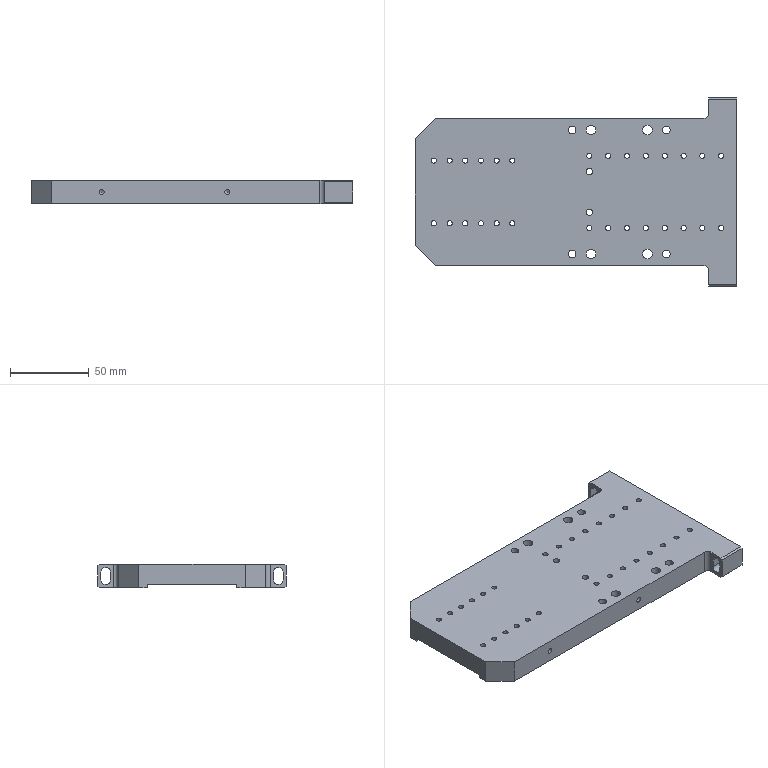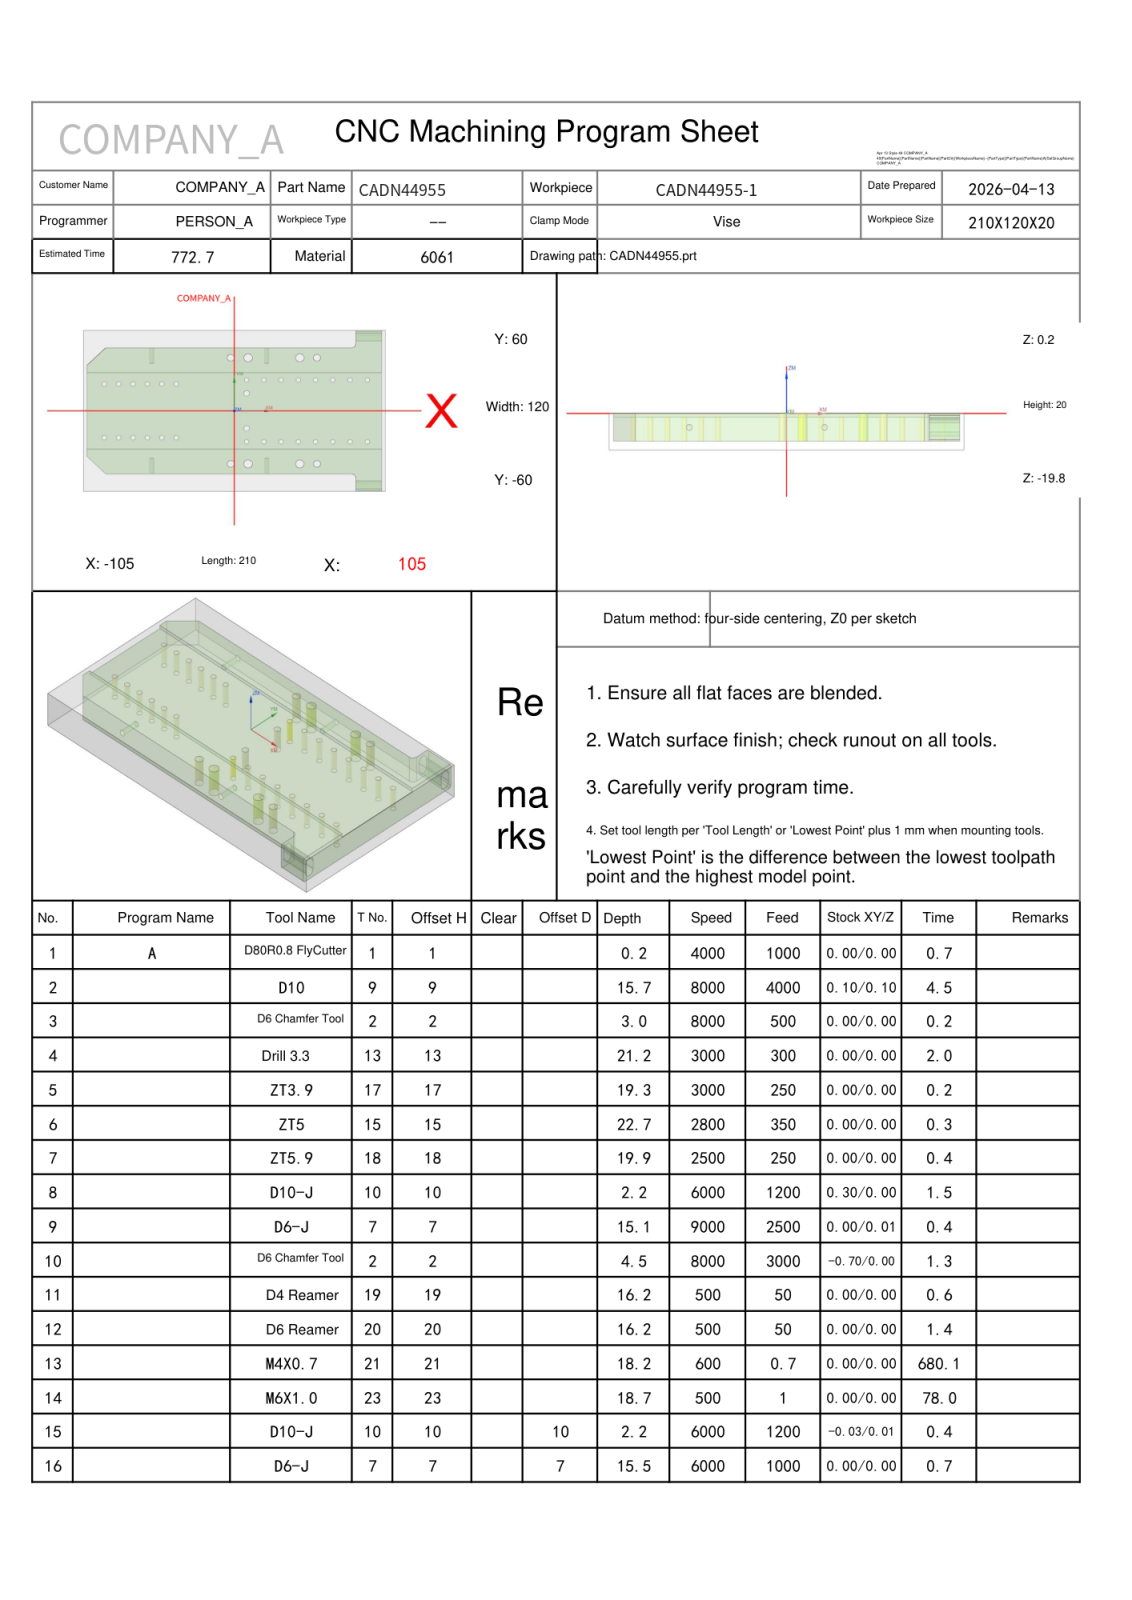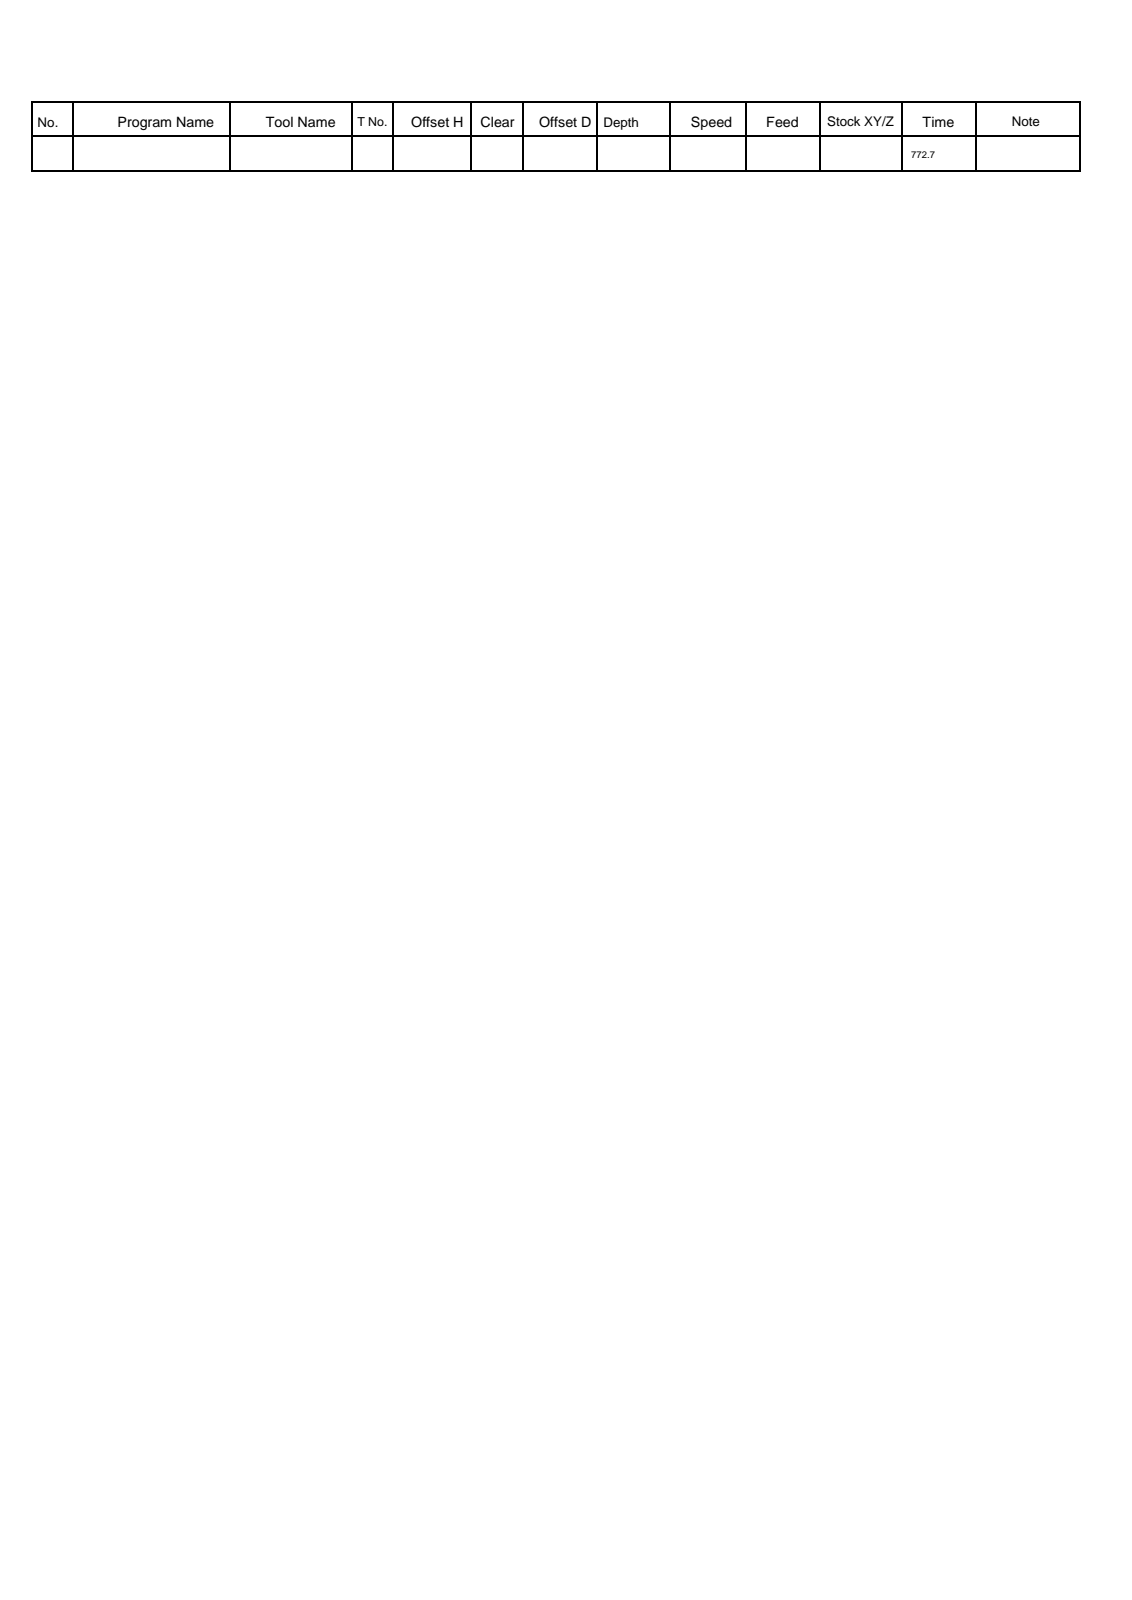NC program | NX | posted by the shop | part box 205 x 120 x 15 mm
Lines 1266 to 2354 of 4760:
N9 T07 M06
(D6-J  D=6. R=0. H=07 ce=0.00 di=0.01)
(MAX_Z=20. MIN_Z=-14.95 Time=0.36M)
G00 G90 G54 X78.684 Y50.9 M03 S9000
G43 H07 Z20.
M08
Z.601
G01 X78.685 Y50.89 Z.472 F2000.
X78.69 Y50.861 Z.356
X78.698 Y50.817 Z.251
X78.71 Y50.759 Z.157
X78.726 Y50.691 Z.073
X78.747 Y50.615 Z0.0
X78.773 Y50.534 Z-.064
X78.804 Y50.45 Z-.119
X78.84 Y50.366 Z-.165
X78.883 Y50.285 Z-.204
X78.932 Y50.209 Z-.235
X78.987 Y50.141 Z-.26
X79.05 Y50.083 Z-.278
X79.12 Y50.039 Z-.29
X79.198 Y50.01 Z-.297
X79.284 Y50. Z-.299
X81.487 F2500.
X81.5
Y52.216
X81.484 Y52.289 Z-.3
X81.437 Y52.343 Z-.303
X81.364 Y52.381 Z-.307
X81.269 Y52.402 Z-.312
X81.155 Y52.41 Z-.319
X81.026 Y52.404 Z-.327
X80.888 Y52.387 Z-.336
X80.742 Y52.359 Z-.346
X80.594 Y52.321 Z-.357
X80.447 Y52.275 Z-.368
X80.306 Y52.222 Z-.38
X80.069 Y52.11 Z-.402
X79.861 Y51.977 Z-.425
X79.679 Y51.821 Z-.449
X79.523 Y51.639 Z-.472
X79.39 Y51.431 Z-.495
X79.278 Y51.194 Z-.517
X79.225 Y51.053 Z-.529
X79.179 Y50.906 Z-.54
X79.141 Y50.758 Z-.551
X79.113 Y50.612 Z-.561
X79.096 Y50.474 Z-.57
X79.09 Y50.345 Z-.578
X79.098 Y50.231 Z-.585
X79.119 Y50.136 Z-.59
X79.157 Y50.063 Z-.594
X79.211 Y50.016 Z-.597
X79.284 Y50. Z-.598
X81.487
X81.5
Y52.216
X81.484 Y52.289 Z-.599
X81.437 Y52.343 Z-.602
X81.364 Y52.381 Z-.606
X81.269 Y52.402 Z-.611
X81.155 Y52.41 Z-.618
X81.026 Y52.404 Z-.626
X80.888 Y52.387 Z-.635
X80.742 Y52.359 Z-.645
X80.594 Y52.321 Z-.656
X80.447 Y52.275 Z-.667
X80.306 Y52.222 Z-.679
X80.069 Y52.11 Z-.701
X79.861 Y51.977 Z-.724
X79.679 Y51.821 Z-.748
X79.523 Y51.639 Z-.771
X79.39 Y51.431 Z-.794
X79.278 Y51.194 Z-.816
X79.225 Y51.053 Z-.828
X79.179 Y50.906 Z-.839
X79.141 Y50.758 Z-.85
X79.113 Y50.612 Z-.86
X79.096 Y50.474 Z-.869
X79.09 Y50.345 Z-.877
X79.098 Y50.231 Z-.884
X79.119 Y50.136 Z-.889
X79.157 Y50.063 Z-.893
X79.211 Y50.016 Z-.896
X79.284 Y50. Z-.897
X81.487
X81.5
Y52.216
X81.484 Y52.289 Z-.898
X81.437 Y52.343 Z-.901
X81.364 Y52.381 Z-.905
X81.269 Y52.402 Z-.91
X81.155 Y52.41 Z-.917
X81.026 Y52.404 Z-.925
X80.888 Y52.387 Z-.934
X80.742 Y52.359 Z-.944
X80.594 Y52.321 Z-.955
X80.447 Y52.275 Z-.966
X80.306 Y52.222 Z-.978
X80.069 Y52.11 Z-1.
X79.861 Y51.977 Z-1.023
X79.679 Y51.821 Z-1.047
X79.523 Y51.639 Z-1.07
X79.39 Y51.431 Z-1.093
X79.278 Y51.194 Z-1.115
X79.225 Y51.053 Z-1.127
X79.179 Y50.906 Z-1.138
X79.141 Y50.758 Z-1.149
X79.113 Y50.612 Z-1.159
X79.096 Y50.474 Z-1.168
X79.09 Y50.345 Z-1.176
X79.098 Y50.231 Z-1.183
X79.119 Y50.136 Z-1.188
X79.157 Y50.063 Z-1.192
X79.211 Y50.016 Z-1.195
X79.284 Y50. Z-1.196
X81.487
X81.5
Y52.216
X81.484 Y52.289 Z-1.197
X81.437 Y52.343 Z-1.2
X81.364 Y52.381 Z-1.204
X81.269 Y52.402 Z-1.209
X81.155 Y52.41 Z-1.216
X81.026 Y52.404 Z-1.224
X80.888 Y52.387 Z-1.233
X80.742 Y52.359 Z-1.243
X80.594 Y52.321 Z-1.254
X80.447 Y52.275 Z-1.265
X80.306 Y52.222 Z-1.277
X80.069 Y52.11 Z-1.299
X79.861 Y51.977 Z-1.322
X79.679 Y51.821 Z-1.346
X79.523 Y51.639 Z-1.369
X79.39 Y51.431 Z-1.392
X79.278 Y51.194 Z-1.414
X79.225 Y51.053 Z-1.426
X79.179 Y50.906 Z-1.437
X79.141 Y50.758 Z-1.448
X79.113 Y50.612 Z-1.458
X79.096 Y50.474 Z-1.467
X79.09 Y50.345 Z-1.475
X79.098 Y50.231 Z-1.482
X79.119 Y50.136 Z-1.487
X79.157 Y50.063 Z-1.491
X79.211 Y50.016 Z-1.494
X79.284 Y50. Z-1.495
X81.487
X81.5
Y52.216
X81.484 Y52.289 Z-1.496
X81.437 Y52.343 Z-1.499
X81.364 Y52.381 Z-1.503
X81.269 Y52.402 Z-1.508
X81.155 Y52.41 Z-1.515
X81.026 Y52.404 Z-1.523
X80.888 Y52.387 Z-1.532
X80.742 Y52.359 Z-1.542
X80.594 Y52.321 Z-1.553
X80.447 Y52.275 Z-1.564
X80.306 Y52.222 Z-1.576
X80.069 Y52.11 Z-1.598
X79.861 Y51.977 Z-1.621
X79.679 Y51.821 Z-1.645
X79.523 Y51.639 Z-1.668
X79.39 Y51.431 Z-1.691
X79.278 Y51.194 Z-1.713
X79.225 Y51.053 Z-1.725
X79.179 Y50.906 Z-1.736
X79.141 Y50.758 Z-1.747
X79.113 Y50.612 Z-1.757
X79.096 Y50.474 Z-1.766
X79.09 Y50.345 Z-1.774
X79.098 Y50.231 Z-1.781
X79.119 Y50.136 Z-1.786
X79.157 Y50.063 Z-1.79
X79.211 Y50.016 Z-1.793
X79.284 Y50. Z-1.794
X81.487
X81.5
Y52.216
X81.484 Y52.289 Z-1.795
X81.437 Y52.343 Z-1.798
X81.364 Y52.381 Z-1.802
X81.269 Y52.402 Z-1.807
X81.155 Y52.41 Z-1.814
X81.026 Y52.404 Z-1.822
X80.888 Y52.387 Z-1.831
X80.742 Y52.359 Z-1.841
X80.594 Y52.321 Z-1.852
X80.447 Y52.275 Z-1.863
X80.306 Y52.222 Z-1.875
X80.069 Y52.11 Z-1.897
X79.861 Y51.977 Z-1.92
X79.679 Y51.821 Z-1.944
X79.523 Y51.639 Z-1.967
X79.39 Y51.431 Z-1.99
X79.278 Y51.194 Z-2.012
X79.225 Y51.053 Z-2.024
X79.179 Y50.906 Z-2.035
X79.141 Y50.758 Z-2.046
X79.113 Y50.612 Z-2.056
X79.096 Y50.474 Z-2.065
X79.09 Y50.345 Z-2.073
X79.098 Y50.231 Z-2.08
X79.119 Y50.136 Z-2.085
X79.157 Y50.063 Z-2.089
X79.211 Y50.016 Z-2.092
X79.284 Y50. Z-2.093
X81.487
X81.5
Y52.216
X81.484 Y52.289 Z-2.094
X81.437 Y52.343 Z-2.097
X81.364 Y52.381 Z-2.101
X81.269 Y52.402 Z-2.106
X81.155 Y52.41 Z-2.113
X81.026 Y52.404 Z-2.121
X80.888 Y52.387 Z-2.13
X80.742 Y52.359 Z-2.14
X80.594 Y52.321 Z-2.151
X80.447 Y52.275 Z-2.162
X80.306 Y52.222 Z-2.174
X80.069 Y52.11 Z-2.196
X79.861 Y51.977 Z-2.219
X79.679 Y51.821 Z-2.243
X79.523 Y51.639 Z-2.266
X79.39 Y51.431 Z-2.289
X79.278 Y51.194 Z-2.311
X79.225 Y51.053 Z-2.323
X79.179 Y50.906 Z-2.334
X79.141 Y50.758 Z-2.345
X79.113 Y50.612 Z-2.355
X79.096 Y50.474 Z-2.364
X79.09 Y50.345 Z-2.372
X79.098 Y50.231 Z-2.379
X79.119 Y50.136 Z-2.384
X79.157 Y50.063 Z-2.388
X79.211 Y50.016 Z-2.391
X79.284 Y50. Z-2.392
X81.487
X81.5
Y52.216
X81.484 Y52.289 Z-2.393
X81.437 Y52.343 Z-2.396
X81.364 Y52.381 Z-2.4
X81.269 Y52.402 Z-2.405
X81.155 Y52.41 Z-2.412
X81.026 Y52.404 Z-2.42
X80.888 Y52.387 Z-2.429
X80.742 Y52.359 Z-2.439
X80.594 Y52.321 Z-2.45
X80.447 Y52.275 Z-2.461
X80.306 Y52.222 Z-2.473
X80.069 Y52.11 Z-2.495
X79.861 Y51.977 Z-2.518
X79.679 Y51.821 Z-2.542
X79.523 Y51.639 Z-2.565
X79.39 Y51.431 Z-2.588
X79.278 Y51.194 Z-2.61
X79.225 Y51.053 Z-2.622
X79.179 Y50.906 Z-2.633
X79.141 Y50.758 Z-2.644
X79.113 Y50.612 Z-2.654
X79.096 Y50.474 Z-2.663
X79.09 Y50.345 Z-2.671
X79.098 Y50.231 Z-2.678
X79.119 Y50.136 Z-2.683
X79.157 Y50.063 Z-2.687
X79.211 Y50.016 Z-2.69
X79.284 Y50. Z-2.691
X81.487
X81.5
Y52.216
X81.484 Y52.289 Z-2.692
X81.437 Y52.343 Z-2.695
X81.364 Y52.381 Z-2.699
X81.269 Y52.402 Z-2.704
X81.155 Y52.41 Z-2.711
X81.026 Y52.404 Z-2.719
X80.888 Y52.387 Z-2.728
X80.742 Y52.359 Z-2.738
X80.594 Y52.321 Z-2.749
X80.447 Y52.275 Z-2.76
X80.306 Y52.222 Z-2.772
X80.069 Y52.11 Z-2.794
X79.861 Y51.977 Z-2.817
X79.679 Y51.821 Z-2.841
X79.523 Y51.639 Z-2.864
X79.39 Y51.431 Z-2.887
X79.278 Y51.194 Z-2.909
X79.225 Y51.053 Z-2.921
X79.179 Y50.906 Z-2.932
X79.141 Y50.758 Z-2.943
X79.113 Y50.612 Z-2.953
X79.096 Y50.474 Z-2.962
X79.09 Y50.345 Z-2.97
X79.098 Y50.231 Z-2.977
X79.119 Y50.136 Z-2.982
X79.157 Y50.063 Z-2.986
X79.211 Y50.016 Z-2.989
X79.284 Y50. Z-2.99
X81.487
X81.5
Y52.216
X81.484 Y52.289 Z-2.991
X81.437 Y52.343 Z-2.994
X81.364 Y52.381 Z-2.998
X81.269 Y52.402 Z-3.003
X81.155 Y52.41 Z-3.01
X81.026 Y52.404 Z-3.018
X80.888 Y52.387 Z-3.027
X80.742 Y52.359 Z-3.037
X80.594 Y52.321 Z-3.048
X80.447 Y52.275 Z-3.059
X80.306 Y52.222 Z-3.071
X80.069 Y52.11 Z-3.093
X79.861 Y51.977 Z-3.116
X79.679 Y51.821 Z-3.14
X79.523 Y51.639 Z-3.163
X79.39 Y51.431 Z-3.186
X79.278 Y51.194 Z-3.208
X79.225 Y51.053 Z-3.22
X79.179 Y50.906 Z-3.231
X79.141 Y50.758 Z-3.242
X79.113 Y50.612 Z-3.252
X79.096 Y50.474 Z-3.261
X79.09 Y50.345 Z-3.269
X79.098 Y50.231 Z-3.276
X79.119 Y50.136 Z-3.281
X79.157 Y50.063 Z-3.285
X79.211 Y50.016 Z-3.288
X79.284 Y50. Z-3.289
X81.487
X81.5
Y52.216
X81.484 Y52.289 Z-3.29
X81.437 Y52.343 Z-3.293
X81.364 Y52.381 Z-3.297
X81.269 Y52.402 Z-3.302
X81.155 Y52.41 Z-3.309
X81.026 Y52.404 Z-3.317
X80.888 Y52.387 Z-3.326
X80.742 Y52.359 Z-3.336
X80.594 Y52.321 Z-3.347
X80.447 Y52.275 Z-3.358
X80.306 Y52.222 Z-3.37
X80.069 Y52.11 Z-3.392
X79.861 Y51.977 Z-3.415
X79.679 Y51.821 Z-3.439
X79.523 Y51.639 Z-3.462
X79.39 Y51.431 Z-3.485
X79.278 Y51.194 Z-3.507
X79.225 Y51.053 Z-3.519
X79.179 Y50.906 Z-3.53
X79.142 Y50.758 Z-3.541
X79.113 Y50.612 Z-3.551
X79.096 Y50.474 Z-3.56
X79.09 Y50.345 Z-3.568
X79.098 Y50.231 Z-3.575
X79.119 Y50.136 Z-3.58
X79.157 Y50.063 Z-3.584
X79.211 Y50.016 Z-3.587
X79.284 Y50. Z-3.588
X81.487
X81.5
Y52.216
X81.484 Y52.289 Z-3.589
X81.437 Y52.343 Z-3.592
X81.364 Y52.381 Z-3.596
X81.269 Y52.402 Z-3.601
X81.155 Y52.41 Z-3.608
X81.026 Y52.404 Z-3.616
X80.888 Y52.387 Z-3.625
X80.742 Y52.359 Z-3.635
X80.594 Y52.321 Z-3.646
X80.447 Y52.275 Z-3.657
X80.306 Y52.222 Z-3.669
X80.069 Y52.11 Z-3.691
X79.861 Y51.977 Z-3.714
X79.679 Y51.821 Z-3.738
X79.523 Y51.639 Z-3.761
X79.39 Y51.431 Z-3.784
X79.278 Y51.194 Z-3.806
X79.225 Y51.053 Z-3.818
X79.179 Y50.906 Z-3.829
X79.141 Y50.758 Z-3.84
X79.113 Y50.612 Z-3.85
X79.096 Y50.474 Z-3.859
X79.09 Y50.345 Z-3.867
X79.098 Y50.231 Z-3.874
X79.119 Y50.136 Z-3.879
X79.157 Y50.063 Z-3.883
X79.211 Y50.016 Z-3.886
X79.284 Y50. Z-3.887
X81.487
X81.5
Y52.216
X81.484 Y52.289 Z-3.888
X81.437 Y52.343 Z-3.891
X81.364 Y52.381 Z-3.895
X81.269 Y52.402 Z-3.9
X81.155 Y52.41 Z-3.907
X81.026 Y52.404 Z-3.915
X80.888 Y52.387 Z-3.924
X80.742 Y52.359 Z-3.934
X80.594 Y52.321 Z-3.945
X80.447 Y52.275 Z-3.956
X80.306 Y52.222 Z-3.968
X80.069 Y52.11 Z-3.99
X79.861 Y51.977 Z-4.013
X79.679 Y51.821 Z-4.037
X79.523 Y51.639 Z-4.06
X79.39 Y51.431 Z-4.083
X79.278 Y51.194 Z-4.105
X79.225 Y51.053 Z-4.117
X79.179 Y50.906 Z-4.128
X79.141 Y50.758 Z-4.139
X79.113 Y50.612 Z-4.149
X79.096 Y50.474 Z-4.158
X79.09 Y50.345 Z-4.166
X79.098 Y50.231 Z-4.173
X79.119 Y50.136 Z-4.178
X79.157 Y50.063 Z-4.182
X79.211 Y50.016 Z-4.185
X79.284 Y50. Z-4.186
X81.487
X81.5
Y52.216
X81.484 Y52.289 Z-4.187
X81.437 Y52.343 Z-4.19
X81.364 Y52.381 Z-4.194
X81.269 Y52.402 Z-4.199
X81.155 Y52.41 Z-4.206
X81.026 Y52.404 Z-4.214
X80.888 Y52.387 Z-4.223
X80.742 Y52.359 Z-4.233
X80.594 Y52.321 Z-4.244
X80.447 Y52.275 Z-4.255
X80.306 Y52.222 Z-4.267
X80.069 Y52.11 Z-4.289
X79.861 Y51.977 Z-4.312
X79.679 Y51.821 Z-4.336
X79.523 Y51.639 Z-4.359
X79.39 Y51.431 Z-4.382
X79.278 Y51.194 Z-4.404
X79.225 Y51.053 Z-4.416
X79.179 Y50.906 Z-4.427
X79.141 Y50.758 Z-4.438
X79.113 Y50.612 Z-4.448
X79.096 Y50.474 Z-4.457
X79.09 Y50.345 Z-4.465
X79.098 Y50.231 Z-4.472
X79.119 Y50.136 Z-4.477
X79.157 Y50.063 Z-4.481
X79.211 Y50.016 Z-4.484
X79.284 Y50. Z-4.485
X81.487
X81.5
Y52.216
X81.484 Y52.289 Z-4.486
X81.437 Y52.343 Z-4.489
X81.364 Y52.381 Z-4.493
X81.269 Y52.402 Z-4.498
X81.155 Y52.41 Z-4.505
X81.026 Y52.404 Z-4.513
X80.888 Y52.387 Z-4.522
X80.742 Y52.359 Z-4.532
X80.594 Y52.321 Z-4.543
X80.447 Y52.275 Z-4.554
X80.306 Y52.222 Z-4.566
X80.069 Y52.11 Z-4.588
X79.861 Y51.977 Z-4.611
X79.679 Y51.821 Z-4.635
X79.523 Y51.639 Z-4.658
X79.39 Y51.431 Z-4.681
X79.278 Y51.194 Z-4.703
X79.225 Y51.053 Z-4.715
X79.179 Y50.906 Z-4.726
X79.141 Y50.758 Z-4.737
X79.113 Y50.612 Z-4.747
X79.096 Y50.474 Z-4.756
X79.09 Y50.345 Z-4.764
X79.098 Y50.231 Z-4.771
X79.119 Y50.136 Z-4.776
X79.157 Y50.063 Z-4.78
X79.211 Y50.016 Z-4.783
X79.284 Y50. Z-4.784
X81.487
X81.5
Y52.216
X81.484 Y52.289 Z-4.785
X81.437 Y52.343 Z-4.788
X81.364 Y52.381 Z-4.792
X81.269 Y52.402 Z-4.797
X81.155 Y52.41 Z-4.804
X81.026 Y52.404 Z-4.812
X80.888 Y52.387 Z-4.821
X80.742 Y52.359 Z-4.831
X80.594 Y52.321 Z-4.842
X80.447 Y52.275 Z-4.853
X80.306 Y52.222 Z-4.865
X80.069 Y52.11 Z-4.887
X79.861 Y51.977 Z-4.91
X79.679 Y51.821 Z-4.934
X79.523 Y51.639 Z-4.957
X79.39 Y51.431 Z-4.98
X79.278 Y51.194 Z-5.002
X79.225 Y51.053 Z-5.014
X79.179 Y50.906 Z-5.025
X79.141 Y50.758 Z-5.036
X79.113 Y50.612 Z-5.046
X79.096 Y50.474 Z-5.055
X79.09 Y50.345 Z-5.063
X79.098 Y50.231 Z-5.07
X79.119 Y50.136 Z-5.075
X79.157 Y50.063 Z-5.079
X79.211 Y50.016 Z-5.082
X79.284 Y50. Z-5.083
X81.487
X81.5
Y52.216
X81.484 Y52.289 Z-5.084
X81.437 Y52.343 Z-5.087
X81.364 Y52.381 Z-5.091
X81.269 Y52.402 Z-5.096
X81.155 Y52.41 Z-5.103
X81.026 Y52.404 Z-5.111
X80.888 Y52.387 Z-5.12
X80.742 Y52.359 Z-5.13
X80.594 Y52.321 Z-5.141
X80.447 Y52.275 Z-5.152
X80.306 Y52.222 Z-5.164
X80.069 Y52.11 Z-5.186
X79.861 Y51.977 Z-5.209
X79.679 Y51.821 Z-5.233
X79.523 Y51.639 Z-5.256
X79.39 Y51.431 Z-5.279
X79.278 Y51.194 Z-5.301
X79.225 Y51.053 Z-5.313
X79.179 Y50.906 Z-5.324
X79.141 Y50.758 Z-5.335
X79.113 Y50.612 Z-5.345
X79.096 Y50.474 Z-5.354
X79.09 Y50.345 Z-5.362
X79.098 Y50.231 Z-5.369
X79.119 Y50.136 Z-5.374
X79.157 Y50.063 Z-5.378
X79.211 Y50.016 Z-5.381
X79.284 Y50. Z-5.382
X81.487
X81.5
Y52.216
X81.484 Y52.289 Z-5.383
X81.437 Y52.343 Z-5.386
X81.364 Y52.381 Z-5.39
X81.269 Y52.402 Z-5.395
X81.155 Y52.41 Z-5.402
X81.026 Y52.404 Z-5.41
X80.888 Y52.387 Z-5.419
X80.742 Y52.359 Z-5.429
X80.594 Y52.321 Z-5.44
X80.447 Y52.275 Z-5.451
X80.306 Y52.222 Z-5.463
X80.069 Y52.11 Z-5.485
X79.861 Y51.977 Z-5.508
X79.679 Y51.821 Z-5.532
X79.523 Y51.639 Z-5.555
X79.39 Y51.431 Z-5.578
X79.278 Y51.194 Z-5.6
X79.225 Y51.053 Z-5.612
X79.179 Y50.906 Z-5.623
X79.141 Y50.758 Z-5.634
X79.113 Y50.612 Z-5.644
X79.096 Y50.474 Z-5.653
X79.09 Y50.345 Z-5.661
X79.098 Y50.231 Z-5.668
X79.119 Y50.136 Z-5.673
X79.157 Y50.063 Z-5.677
X79.211 Y50.016 Z-5.68
X79.284 Y50. Z-5.681
X81.487
X81.5
Y52.216
X81.484 Y52.289 Z-5.682
X81.437 Y52.343 Z-5.685
X81.364 Y52.381 Z-5.689
X81.269 Y52.402 Z-5.694
X81.155 Y52.41 Z-5.701
X81.026 Y52.404 Z-5.709
X80.888 Y52.387 Z-5.718
X80.742 Y52.359 Z-5.728
X80.594 Y52.321 Z-5.739
X80.447 Y52.275 Z-5.75
X80.306 Y52.222 Z-5.762
X80.069 Y52.11 Z-5.784
X79.861 Y51.977 Z-5.807
X79.679 Y51.821 Z-5.831
X79.523 Y51.639 Z-5.854
X79.39 Y51.431 Z-5.877
X79.278 Y51.194 Z-5.899
X79.225 Y51.053 Z-5.911
X79.179 Y50.906 Z-5.922
X79.141 Y50.758 Z-5.933
X79.113 Y50.612 Z-5.943
X79.096 Y50.474 Z-5.952
X79.09 Y50.345 Z-5.96
X79.098 Y50.231 Z-5.967
X79.119 Y50.136 Z-5.972
X79.157 Y50.063 Z-5.976
X79.211 Y50.016 Z-5.979
X79.284 Y50. Z-5.98
X81.487
X81.5
Y52.216
X81.484 Y52.289 Z-5.981
X81.437 Y52.343 Z-5.984
X81.364 Y52.381 Z-5.988
X81.269 Y52.402 Z-5.993
X81.155 Y52.41 Z-6.
X81.026 Y52.404 Z-6.008
X80.888 Y52.387 Z-6.017
X80.742 Y52.359 Z-6.027
X80.594 Y52.321 Z-6.038
X80.447 Y52.275 Z-6.049
X80.306 Y52.222 Z-6.061
X80.069 Y52.11 Z-6.083
X79.861 Y51.977 Z-6.106
X79.679 Y51.821 Z-6.13
X79.523 Y51.639 Z-6.153
X79.39 Y51.431 Z-6.176
X79.278 Y51.194 Z-6.198
X79.225 Y51.053 Z-6.21
X79.179 Y50.906 Z-6.221
X79.141 Y50.758 Z-6.232
X79.113 Y50.612 Z-6.242
X79.096 Y50.474 Z-6.251
X79.09 Y50.345 Z-6.259
X79.098 Y50.231 Z-6.266
X79.119 Y50.136 Z-6.271
X79.157 Y50.063 Z-6.275
X79.211 Y50.016 Z-6.278
X79.284 Y50. Z-6.279
X81.487
X81.5
Y52.216
X81.484 Y52.289 Z-6.28
X81.437 Y52.343 Z-6.283
X81.364 Y52.381 Z-6.287
X81.269 Y52.402 Z-6.292
X81.155 Y52.41 Z-6.299
X81.026 Y52.404 Z-6.307
X80.888 Y52.387 Z-6.316
X80.742 Y52.359 Z-6.326
X80.594 Y52.321 Z-6.337
X80.447 Y52.275 Z-6.348
X80.306 Y52.222 Z-6.36
X80.069 Y52.11 Z-6.382
X79.861 Y51.977 Z-6.405
X79.679 Y51.821 Z-6.429
X79.523 Y51.639 Z-6.452
X79.39 Y51.431 Z-6.475
X79.278 Y51.194 Z-6.497
X79.225 Y51.053 Z-6.509
X79.179 Y50.906 Z-6.52
X79.141 Y50.758 Z-6.531
X79.113 Y50.612 Z-6.541
X79.096 Y50.474 Z-6.55
X79.09 Y50.345 Z-6.558
X79.098 Y50.231 Z-6.565
X79.119 Y50.136 Z-6.57
X79.157 Y50.063 Z-6.574
X79.211 Y50.016 Z-6.577
X79.284 Y50. Z-6.578
X81.487
X81.5
Y52.216
X81.484 Y52.289 Z-6.579
X81.437 Y52.343 Z-6.582
X81.364 Y52.381 Z-6.586
X81.269 Y52.402 Z-6.591
X81.155 Y52.41 Z-6.598
X81.026 Y52.404 Z-6.606
X80.888 Y52.387 Z-6.615
X80.742 Y52.359 Z-6.625
X80.594 Y52.321 Z-6.636
X80.447 Y52.275 Z-6.647
X80.306 Y52.222 Z-6.659
X80.069 Y52.11 Z-6.681
X79.861 Y51.977 Z-6.704
X79.679 Y51.821 Z-6.728
X79.523 Y51.639 Z-6.751
X79.39 Y51.431 Z-6.774
X79.278 Y51.194 Z-6.796
X79.225 Y51.053 Z-6.808
X79.179 Y50.906 Z-6.819
X79.141 Y50.758 Z-6.83
X79.113 Y50.612 Z-6.84
X79.096 Y50.474 Z-6.849
X79.09 Y50.345 Z-6.857
X79.098 Y50.231 Z-6.864
X79.119 Y50.136 Z-6.869
X79.157 Y50.063 Z-6.873
X79.211 Y50.016 Z-6.876
X79.284 Y50. Z-6.877
X81.487
X81.5
Y52.216
X81.484 Y52.289 Z-6.878
X81.437 Y52.343 Z-6.881
X81.364 Y52.381 Z-6.885
X81.269 Y52.402 Z-6.89
X81.155 Y52.41 Z-6.897
X81.026 Y52.404 Z-6.905
X80.888 Y52.387 Z-6.914
X80.742 Y52.359 Z-6.924
X80.594 Y52.321 Z-6.935
X80.447 Y52.275 Z-6.946
X80.306 Y52.222 Z-6.958
X80.069 Y52.11 Z-6.98
X79.861 Y51.977 Z-7.003
X79.679 Y51.821 Z-7.027
X79.523 Y51.639 Z-7.05
X79.39 Y51.431 Z-7.073
X79.278 Y51.194 Z-7.095
X79.225 Y51.053 Z-7.107
X79.179 Y50.906 Z-7.118
X79.141 Y50.758 Z-7.129
X79.113 Y50.612 Z-7.139
X79.096 Y50.474 Z-7.148
X79.09 Y50.345 Z-7.156
X79.098 Y50.231 Z-7.163
X79.119 Y50.136 Z-7.168
X79.157 Y50.063 Z-7.172
X79.211 Y50.016 Z-7.175
X79.284 Y50. Z-7.176
X81.487
X81.5
Y52.216
X81.484 Y52.289 Z-7.177
X81.437 Y52.343 Z-7.18
X81.364 Y52.381 Z-7.184
X81.269 Y52.402 Z-7.189
X81.155 Y52.41 Z-7.196
X81.026 Y52.404 Z-7.204
X80.888 Y52.387 Z-7.213
X80.742 Y52.359 Z-7.223
X80.594 Y52.321 Z-7.234
X80.447 Y52.275 Z-7.245
X80.306 Y52.222 Z-7.257
X80.069 Y52.11 Z-7.279
X79.861 Y51.977 Z-7.302
X79.679 Y51.821 Z-7.326
X79.523 Y51.639 Z-7.349
X79.39 Y51.431 Z-7.372
X79.278 Y51.194 Z-7.394
X79.225 Y51.053 Z-7.406
X79.179 Y50.906 Z-7.417
X79.141 Y50.758 Z-7.428
X79.113 Y50.612 Z-7.438
X79.096 Y50.474 Z-7.447
X79.09 Y50.345 Z-7.455
X79.098 Y50.231 Z-7.462
X79.119 Y50.136 Z-7.467
X79.157 Y50.063 Z-7.471
X79.211 Y50.016 Z-7.474
X79.284 Y50. Z-7.475
X81.487
X81.5
Y52.216
X81.484 Y52.289 Z-7.476
X81.437 Y52.343 Z-7.479
X81.364 Y52.381 Z-7.483
X81.269 Y52.402 Z-7.488
X81.155 Y52.41 Z-7.495
X81.026 Y52.404 Z-7.503
X80.888 Y52.387 Z-7.512
X80.742 Y52.359 Z-7.522
X80.594 Y52.321 Z-7.533
X80.447 Y52.275 Z-7.544
X80.306 Y52.222 Z-7.556
X80.069 Y52.11 Z-7.578
X79.861 Y51.977 Z-7.601
X79.679 Y51.821 Z-7.625
X79.523 Y51.639 Z-7.648
X79.39 Y51.431 Z-7.671
X79.278 Y51.194 Z-7.693
X79.225 Y51.053 Z-7.705
X79.179 Y50.906 Z-7.716
X79.142 Y50.758 Z-7.727
X79.113 Y50.612 Z-7.737
X79.096 Y50.474 Z-7.746
X79.09 Y50.345 Z-7.754
X79.098 Y50.231 Z-7.761
X79.119 Y50.136 Z-7.766
X79.157 Y50.063 Z-7.77
X79.211 Y50.016 Z-7.773
X79.284 Y50. Z-7.774
X81.487
X81.5
Y52.216
X81.484 Y52.289 Z-7.775
X81.437 Y52.343 Z-7.778
X81.364 Y52.381 Z-7.782
X81.269 Y52.402 Z-7.787
X81.155 Y52.41 Z-7.794
X81.026 Y52.404 Z-7.802
X80.888 Y52.387 Z-7.811
X80.742 Y52.359 Z-7.821
X80.594 Y52.321 Z-7.832
X80.447 Y52.275 Z-7.843
X80.306 Y52.222 Z-7.855
X80.069 Y52.11 Z-7.877
X79.861 Y51.977 Z-7.9
X79.679 Y51.821 Z-7.924
X79.523 Y51.639 Z-7.947
X79.39 Y51.431 Z-7.97
X79.278 Y51.194 Z-7.992
X79.225 Y51.053 Z-8.004
X79.179 Y50.906 Z-8.015
X79.142 Y50.758 Z-8.026
X79.113 Y50.612 Z-8.036
X79.096 Y50.474 Z-8.045
X79.09 Y50.345 Z-8.053
X79.098 Y50.231 Z-8.06
X79.119 Y50.136 Z-8.065
X79.157 Y50.063 Z-8.069
X79.211 Y50.016 Z-8.072
X79.284 Y50. Z-8.073
X81.487
X81.5
Y52.216
X81.484 Y52.289 Z-8.074
X81.437 Y52.343 Z-8.077
X81.364 Y52.381 Z-8.081
X81.269 Y52.402 Z-8.086
X81.155 Y52.41 Z-8.093
X81.026 Y52.404 Z-8.101
X80.888 Y52.387 Z-8.11
X80.742 Y52.359 Z-8.12
X80.594 Y52.321 Z-8.131
X80.447 Y52.275 Z-8.142
X80.306 Y52.222 Z-8.154
X80.069 Y52.11 Z-8.176
X79.861 Y51.977 Z-8.199
X79.679 Y51.821 Z-8.223
X79.523 Y51.639 Z-8.246
X79.39 Y51.431 Z-8.269
X79.278 Y51.194 Z-8.291
X79.225 Y51.053 Z-8.303
X79.179 Y50.906 Z-8.314
X79.142 Y50.758 Z-8.325
X79.113 Y50.612 Z-8.335
X79.096 Y50.474 Z-8.344
X79.09 Y50.345 Z-8.352
X79.098 Y50.231 Z-8.359
X79.119 Y50.136 Z-8.364
X79.157 Y50.063 Z-8.368
X79.211 Y50.016 Z-8.371
X79.284 Y50. Z-8.372
X81.487
X81.5
Y52.216
X81.484 Y52.289 Z-8.373
X81.437 Y52.343 Z-8.376
X81.364 Y52.381 Z-8.38
X81.269 Y52.402 Z-8.385
X81.155 Y52.41 Z-8.392
X81.026 Y52.404 Z-8.4
X80.888 Y52.387 Z-8.409
X80.742 Y52.359 Z-8.419
X80.594 Y52.321 Z-8.43
X80.447 Y52.275 Z-8.441
X80.306 Y52.222 Z-8.453
X80.069 Y52.11 Z-8.475
X79.861 Y51.977 Z-8.498
X79.679 Y51.821 Z-8.522
X79.523 Y51.639 Z-8.545
X79.39 Y51.431 Z-8.568
X79.278 Y51.194 Z-8.59
X79.225 Y51.053 Z-8.602
X79.179 Y50.906 Z-8.613
X79.142 Y50.758 Z-8.624
X79.113 Y50.612 Z-8.634
X79.096 Y50.474 Z-8.643
X79.09 Y50.345 Z-8.651
X79.098 Y50.231 Z-8.658
X79.119 Y50.136 Z-8.663
X79.157 Y50.063 Z-8.667
X79.211 Y50.016 Z-8.67
X79.284 Y50. Z-8.671
X81.487
X81.5
Y52.216
X81.484 Y52.289 Z-8.672
X81.437 Y52.343 Z-8.675
X81.364 Y52.381 Z-8.679
X81.269 Y52.402 Z-8.684
X81.155 Y52.41 Z-8.691
X81.026 Y52.404 Z-8.699
X80.888 Y52.387 Z-8.708
X80.742 Y52.359 Z-8.718
X80.594 Y52.321 Z-8.729
X80.447 Y52.275 Z-8.74
X80.306 Y52.222 Z-8.752
X80.069 Y52.11 Z-8.774
X79.861 Y51.977 Z-8.797
X79.679 Y51.821 Z-8.821
X79.523 Y51.639 Z-8.844
X79.39 Y51.431 Z-8.867
X79.278 Y51.194 Z-8.889
X79.225 Y51.053 Z-8.901
X79.179 Y50.906 Z-8.912
X79.142 Y50.758 Z-8.923
X79.113 Y50.612 Z-8.933
X79.096 Y50.474 Z-8.942
X79.09 Y50.345 Z-8.95
X79.098 Y50.231 Z-8.957
X79.119 Y50.136 Z-8.962
X79.157 Y50.063 Z-8.966
X79.211 Y50.016 Z-8.969
X79.284 Y50. Z-8.97
X81.487
X81.5
Y52.216
X81.484 Y52.289 Z-8.971
X81.437 Y52.343 Z-8.974
X81.364 Y52.381 Z-8.978
X81.269 Y52.402 Z-8.983
X81.155 Y52.41 Z-8.99
X81.026 Y52.404 Z-8.998
X80.888 Y52.387 Z-9.007
X80.742 Y52.359 Z-9.017
X80.594 Y52.321 Z-9.028
X80.447 Y52.275 Z-9.039
X80.306 Y52.222 Z-9.051
X80.069 Y52.11 Z-9.073
X79.861 Y51.977 Z-9.096
X79.679 Y51.821 Z-9.12
X79.523 Y51.639 Z-9.143
X79.39 Y51.431 Z-9.166
X79.278 Y51.194 Z-9.188
X79.225 Y51.053 Z-9.2
X79.179 Y50.906 Z-9.211
X79.142 Y50.758 Z-9.222
X79.113 Y50.612 Z-9.232
X79.096 Y50.474 Z-9.241
X79.09 Y50.345 Z-9.249
X79.098 Y50.231 Z-9.256
X79.119 Y50.136 Z-9.261
X79.157 Y50.063 Z-9.265
X79.211 Y50.016 Z-9.268
X79.284 Y50. Z-9.269
X81.487
X81.5
Y52.216
X81.484 Y52.289 Z-9.27
X81.437 Y52.343 Z-9.273
X81.364 Y52.381 Z-9.277
X81.269 Y52.402 Z-9.282
X81.155 Y52.41 Z-9.289
X81.026 Y52.404 Z-9.297
X80.888 Y52.387 Z-9.306
X80.742 Y52.359 Z-9.316
X80.594 Y52.321 Z-9.327
X80.447 Y52.275 Z-9.338
X80.306 Y52.222 Z-9.35
X80.069 Y52.11 Z-9.372
X79.861 Y51.977 Z-9.395
X79.679 Y51.821 Z-9.419
X79.523 Y51.639 Z-9.442
X79.39 Y51.431 Z-9.465
X79.278 Y51.194 Z-9.487
X79.225 Y51.053 Z-9.499
X79.179 Y50.906 Z-9.51
X79.142 Y50.758 Z-9.521
X79.113 Y50.612 Z-9.531
X79.096 Y50.474 Z-9.54
X79.09 Y50.345 Z-9.548
X79.098 Y50.231 Z-9.555
X79.119 Y50.136 Z-9.56
X79.157 Y50.063 Z-9.564
X79.211 Y50.016 Z-9.567
X79.284 Y50. Z-9.568
X81.487
X81.5
Y52.216
X81.484 Y52.289 Z-9.569
X81.437 Y52.343 Z-9.572
X81.364 Y52.381 Z-9.576
X81.269 Y52.402 Z-9.581
X81.155 Y52.41 Z-9.588
X81.026 Y52.404 Z-9.596
X80.888 Y52.387 Z-9.605
X80.742 Y52.359 Z-9.615
X80.594 Y52.321 Z-9.626
X80.447 Y52.275 Z-9.637
X80.306 Y52.222 Z-9.649
X80.069 Y52.11 Z-9.671
X79.861 Y51.977 Z-9.694
X79.679 Y51.821 Z-9.718
X79.523 Y51.639 Z-9.741
X79.39 Y51.431 Z-9.764
X79.278 Y51.194 Z-9.786
X79.225 Y51.053 Z-9.798
X79.179 Y50.906 Z-9.809
X79.142 Y50.758 Z-9.82
X79.113 Y50.612 Z-9.83
X79.096 Y50.474 Z-9.839
X79.09 Y50.345 Z-9.847
X79.098 Y50.231 Z-9.854
X79.119 Y50.136 Z-9.859
X79.157 Y50.063 Z-9.863
X79.211 Y50.016 Z-9.866
X79.284 Y50. Z-9.867
X81.487
X81.5
Y52.216
X81.484 Y52.289 Z-9.868
X81.437 Y52.343 Z-9.871
X81.364 Y52.381 Z-9.875
X81.269 Y52.402 Z-9.88
X81.155 Y52.41 Z-9.887
X81.026 Y52.404 Z-9.895
X80.888 Y52.387 Z-9.904
X80.742 Y52.359 Z-9.914
X80.594 Y52.321 Z-9.925
X80.447 Y52.275 Z-9.936
X80.306 Y52.222 Z-9.948
X80.069 Y52.11 Z-9.97
X79.861 Y51.977 Z-9.993
X79.679 Y51.821 Z-10.017
X79.523 Y51.639 Z-10.04
X79.39 Y51.431 Z-10.063
X79.278 Y51.194 Z-10.085
X79.225 Y51.053 Z-10.097
X79.179 Y50.906 Z-10.108
X79.142 Y50.758 Z-10.119
X79.113 Y50.612 Z-10.129
X79.096 Y50.474 Z-10.138
X79.09 Y50.345 Z-10.146
X79.098 Y50.231 Z-10.153
X79.119 Y50.136 Z-10.158
X79.157 Y50.063 Z-10.162
X79.211 Y50.016 Z-10.165
X79.284 Y50. Z-10.166
X81.487
X81.5
Y52.216
X81.484 Y52.289 Z-10.167
X81.437 Y52.343 Z-10.17
X81.364 Y52.381 Z-10.174
X81.269 Y52.402 Z-10.179
X81.155 Y52.41 Z-10.186
X81.026 Y52.404 Z-10.194
X80.888 Y52.387 Z-10.203
X80.742 Y52.359 Z-10.213
X80.594 Y52.321 Z-10.224
X80.447 Y52.275 Z-10.235
X80.306 Y52.222 Z-10.247
X80.069 Y52.11 Z-10.269
X79.861 Y51.977 Z-10.292
X79.679 Y51.821 Z-10.316
X79.523 Y51.639 Z-10.339
X79.39 Y51.431 Z-10.362
X79.278 Y51.194 Z-10.384
X79.225 Y51.053 Z-10.396
X79.179 Y50.906 Z-10.407
X79.142 Y50.758 Z-10.418
X79.113 Y50.612 Z-10.428
X79.096 Y50.474 Z-10.437
X79.09 Y50.345 Z-10.445
X79.098 Y50.231 Z-10.452
X79.119 Y50.136 Z-10.457
X79.157 Y50.063 Z-10.461
X79.211 Y50.016 Z-10.464
X79.284 Y50. Z-10.465
X81.487
X81.5
Y52.216
X81.484 Y52.289 Z-10.466
X81.437 Y52.343 Z-10.469
X81.364 Y52.381 Z-10.473
X81.269 Y52.402 Z-10.478
X81.155 Y52.41 Z-10.485
X81.026 Y52.404 Z-10.493
X80.888 Y52.387 Z-10.502
X80.742 Y52.359 Z-10.512
X80.594 Y52.321 Z-10.523